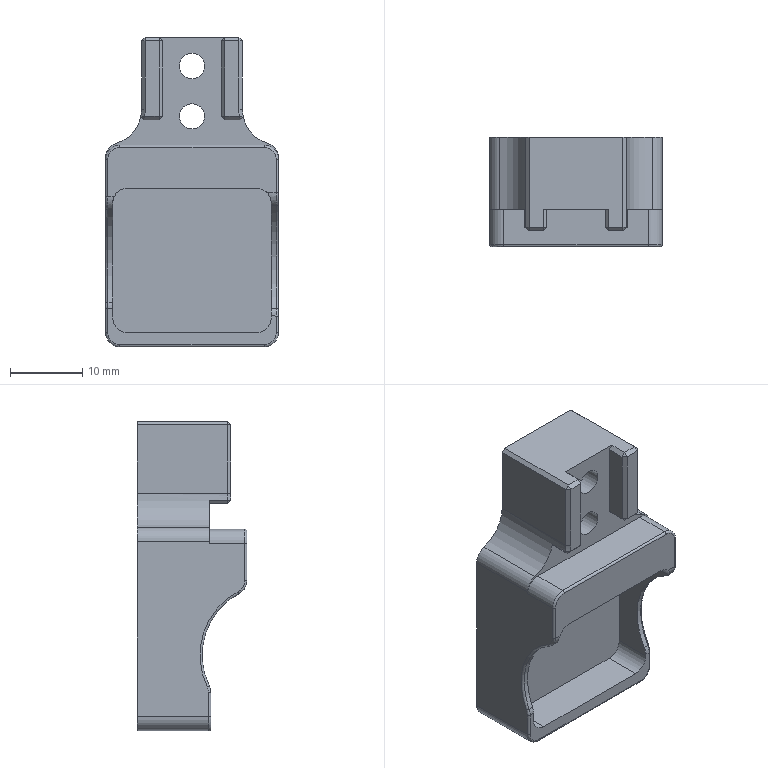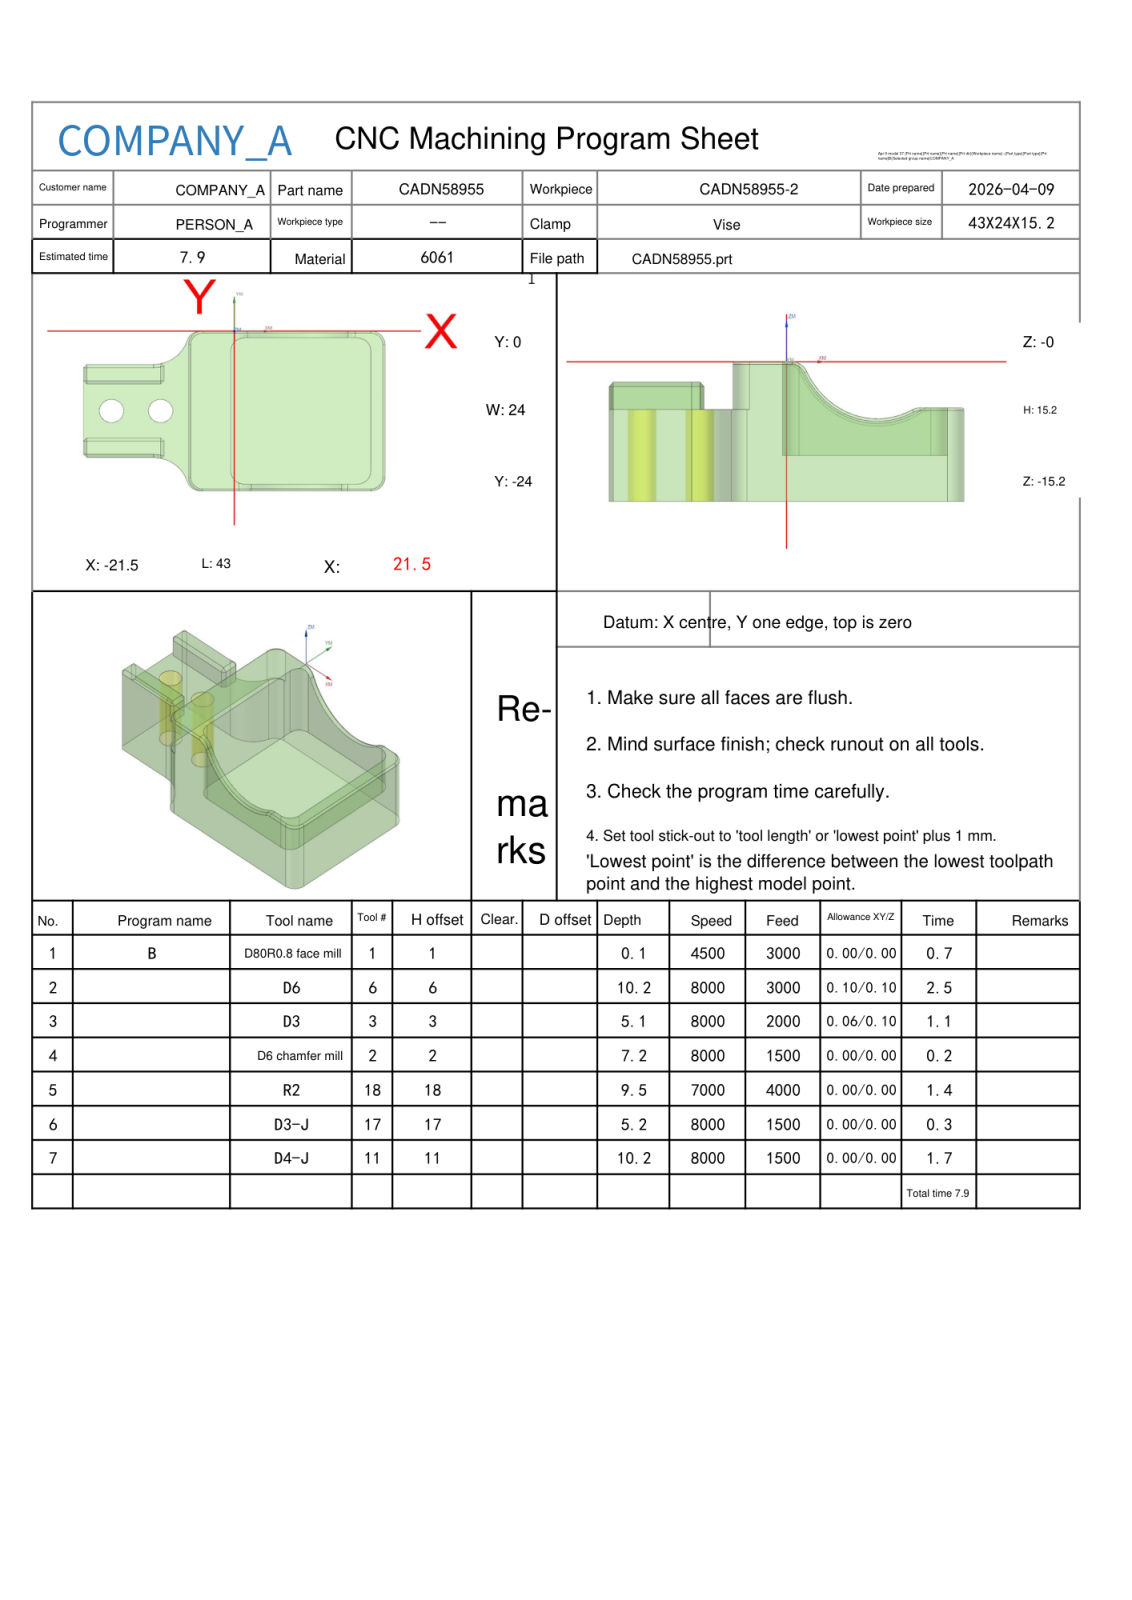NC program | NX | posted by the shop | part box 24 x 15.2 x 43 mm
Lines 1 to 2342 of 14472, first 1929 of 2340 lines:
%
O0001
(Machine time: 9.20 MIN)
(===Total Tool:7===)
(T1=D80R0.8 face mill D=80.  R=0.8  D-  H01 Z=-0.   )
(T6=D6      D=6.   R=0.   D-  H06 Z=-10.2 )
(T3=D3      D=3.   R=0.   D-  H03 Z=-5.1  )
(T2=D6 chamfer mill   D=6.   R=0.   D-  H02 Z=-7.25 )
(T18=R2     D=4.   R=2.   D-  H18 Z=-9.45 )
(T17=D3-J   D=3.   R=0.   D17 H17 Z=-5.2  )
(T11=D4-J   D=4.   R=0.   D11 H11 Z=-10.2 )
G80 G90 G17 G49 G40
G91 G28 Z0
M01
N1 T01 M06
(D80R0.8 face mill D=80. R=0.8 H=01 ce=0.20 di=0.10)
G00 G90 G54 X73.5 Y-12. M03 S4500
G43 H01 Z20.
M08
Z6.011
G01 Z4.011 F3000.
X61.5
X-61.5
X-73.5
Z6.011
G00 Z7.5
X73.5
Z5.522
G01 Z3.522
X61.5
X-61.5
X-73.5
Z5.522
G00 Z7.011
X73.5
Z5.033
G01 Z3.033
X61.5
X-61.5
X-73.5
Z5.033
G00 Z6.522
X73.5
Z4.544
G01 Z2.544
X61.5
X-61.5
X-73.5
Z4.544
G00 Z6.033
X73.5
Z4.056
G01 Z2.056
X61.5
X-61.5
X-73.5
Z4.056
G00 Z5.544
X73.5
Z3.567
G01 Z1.567
X61.5
X-61.5
X-73.5
Z3.567
G00 Z5.056
X73.5
Z3.078
G01 Z1.078
X61.5
X-61.5
X-73.5
Z3.078
G00 Z4.567
X73.5
Z2.589
G01 Z.589
X61.5
X-61.5
X-73.5
Z2.589
G00 Z4.078
X73.5
Z2.1
G01 Z.1
X61.5
X-61.5
X-73.5
Z2.1
G00 Z20.
G00 G90 X73.5 Y-12. M03 S4500
Z20.
Z2.
G01 Z0.0 F1000.
X61.5
X-61.5
X-73.5
Z2.
G00 Z20.
G91 G28 Z0.0
M05
M09
G91 G28 Z0.0
M01
N2 T06 M06
(D6  D=6. R=0. H=06 ce=0.10 di=0.10)
G00 G90 G54 X-23.1 Y.5 M03 S8000
G43 H06 Z14.5
M08
Z1.32
G01 Z-.18 F3000.
Y-2.56
Y-20.84
G03 X-22.5 Y-21.44 I.6 J0.0
G01 X-19.2
G03 X-18.6 Y-20.84 I0.0 J.6
G01 Y-3.16
G02 X-18. Y-2.56 I.6 J0.0
G01 X-14.7
G02 X-14.1 Y-3.16 I0.0 J-.6
G01 Y-20.84
G03 X-13.5 Y-21.44 I.6 J0.0
G01 X-11.5
G02 X-11.034 Y-21.483 I0.0 J-2.56
G01 X-10.724 Y-22.04
G03 X-10.2 Y-22.348 I.524 J.292
X-9.6 Y-21.748 I0.0 J.6
G01 Y-2.252
Y4.261
Z1.32
G00 X-23.1 Y.5
Z.84
G01 Z-.66
Y-2.56
Y-20.84
G03 X-22.5 Y-21.44 I.6 J0.0
G01 X-19.2
G03 X-18.6 Y-20.84 I0.0 J.6
G01 Y-3.16
G02 X-18. Y-2.56 I.6 J0.0
G01 X-14.7
G02 X-14.1 Y-3.16 I0.0 J-.6
G01 Y-20.84
G03 X-13.5 Y-21.44 I.6 J0.0
G01 X-11.5
G02 X-11.034 Y-21.483 I0.0 J-2.56
G01 X-10.724 Y-22.04
G03 X-10.2 Y-22.348 I.524 J.292
X-9.6 Y-21.748 I0.0 J.6
G01 Y-2.252
Y4.293
Z.84
G00 X-23.1 Y.5
Z.36
G01 Z-1.14
Y-2.56
Y-20.84
G03 X-22.5 Y-21.44 I.6 J0.0
G01 X-19.2
G03 X-18.6 Y-20.84 I0.0 J.6
G01 Y-3.16
G02 X-18. Y-2.56 I.6 J0.0
G01 X-14.7
G02 X-14.1 Y-3.16 I0.0 J-.6
G01 Y-20.84
G03 X-13.5 Y-21.44 I.6 J0.0
G01 X-11.5
G02 X-11.034 Y-21.483 I0.0 J-2.56
G01 X-10.724 Y-22.04
G03 X-10.2 Y-22.348 I.524 J.292
X-9.6 Y-21.748 I0.0 J.6
G01 Y-2.252
Y4.293
Z.36
G00 X-23.1 Y.5
Z-.12
G01 Z-1.62
Y-2.56
Y-20.84
G03 X-22.5 Y-21.44 I.6 J0.0
G01 X-19.2
G03 X-18.6 Y-20.84 I0.0 J.6
G01 Y-3.16
G02 X-18. Y-2.56 I.6 J0.0
G01 X-14.7
G02 X-14.1 Y-3.16 I0.0 J-.6
G01 Y-20.84
G03 X-13.5 Y-21.44 I.6 J0.0
G01 X-11.5
G02 X-11.034 Y-21.483 I0.0 J-2.56
G01 X-10.724 Y-22.04
G03 X-10.2 Y-22.348 I.524 J.292
X-9.6 Y-21.748 I0.0 J.6
G01 Y-2.252
Y4.293
Z-.12
G00 X-23.1 Y.5
Z-.6
G01 Z-2.1
Y-2.56
Y-20.84
G03 X-22.5 Y-21.44 I.6 J0.0
G01 X-19.2
G03 X-18.6 Y-20.84 I0.0 J.6
G01 Y-3.16
G02 X-18. Y-2.56 I.6 J0.0
G01 X-14.7
G02 X-14.1 Y-3.16 I0.0 J-.6
G01 Y-20.84
G03 X-13.5 Y-21.44 I.6 J0.0
G01 X-11.5
G02 X-11.034 Y-21.483 I0.0 J-2.56
G01 X-10.724 Y-22.04
G03 X-10.2 Y-22.348 I.524 J.292
X-9.6 Y-21.748 I0.0 J.6
G01 Y-2.252
Y4.293
Z-.6
G00 Z14.5
G00 G90 X28.93 Y-7.803 M03 S8000
Z14.5
Z5.21
G01 Z4.01 F3000.
X28.499
G03 X24.299 Y-12.002 I0.0 J-4.2
G01 X24.297 Y-23.996
G02 X23.868 Y-24.798 I-4.925 J2.121
G01 X23.164 Y-24.8
X1.594 Y-24.798
Y-26.478
X1.595 Y-26.838
X.755 Y-26.839
X.754 Y-26.479
Y-23.719
X.734 Y-22.879
X.754 Y-22.876
X.829 Y-22.88
X.861 Y-22.81
X.81 Y-22.755
X.785 Y-22.715
X1.562 Y-21.053
X1.988 Y-20.803
X2.414 Y-20.579
X2.487 Y-20.558
X2.457 Y-20.488
X2.512 Y-20.469
X2.56 Y-20.476
X2.618 Y-20.508
X2.636 Y-20.445
X2.682 Y-20.38
X2.73 Y-20.255
X2.731 Y-20.048
X2.73 Y-19.928
Y-4.295
X2.732 Y-3.633
X2.796 Y-3.5
X2.814 Y-3.422
X2.735 Y-3.414
X2.654 Y-3.395
X2.637 Y-3.374
X2.623 Y-3.315
X2.569 Y-3.345
X2.58 Y-3.284
X2.518 Y-3.29
X2.462 Y-3.272
X2.397 Y-3.262
X1.551 Y-2.938
X.332 Y-1.642
X.381 Y-1.622
X.432 Y-1.548
X.362 Y-1.468
X.254 Y-1.457
X.208 Y-1.459
X.187 Y-.619
X.179 Y-.278
Y2.479
Y2.839
X1.019 Y2.838
Y2.479
Y.797
X23.891
G02 X24.299 Y.029 I-4.506 J-2.886
G01 X24.3 Y-.364
X24.298 Y-13.194
G02 X24.047 Y-13.682 I-.6 J0.0
G01 X20.349 Y-16.322
G03 X20.098 Y-16.81 I.349 J-.488
G01 Y-20.
G02 X19.498 Y-20.599 I-.6 J.001
G01 X7.53
G02 X6.931 Y-20.006 I.001 J.6
G01 X6.93 Y-19.907
Y-4.295
X6.938 Y-4.197
G03 X6.973 Y-3.939 I-4.221 J.706
G02 X7.569 Y-3.403 I.597 J-.064
G01 X19.5
G02 X20.1 Y-4.002 I-.001 J-.6
G01 X20.098 Y-13.146
G02 X19.787 Y-13.672 I-.6 J0.0
G01 X16.144 Y-15.666
G03 X15.865 Y-15.996 I.288 J-.526
G02 X15.299 Y-16.399 I-.567 J.196
G01 X11.729
G02 X11.13 Y-15.8 I.001 J.6
G01 Y-8.202
G02 X11.729 Y-7.603 I.6 J-.001
G01 X15.3
G02 X15.899 Y-8.202 I-.001 J-.6
G01 X15.898 Y-15.001
Y-15.501
G03 X20.098 Y-19.702 I4.2 J0.0
G01 X28.93 Y-19.703
Z5.21
G00 Z7.5
G01 Y-7.803 F6000.
G00 Z4.72
G01 Z3.52 F3000.
X28.499
G03 X24.299 Y-12.002 I0.0 J-4.2
G01 X24.297 Y-23.996
G02 X23.868 Y-24.798 I-4.925 J2.12
G01 X23.164 Y-24.8
X1.594 Y-24.799
Y-26.478
X1.595 Y-26.838
X.755 Y-26.839
X.754 Y-26.479
Y-23.719
X.734 Y-22.879
X.754 Y-22.876
X.829 Y-22.88
X.861 Y-22.81
X.81 Y-22.755
X.785 Y-22.715
X1.562 Y-21.053
X1.988 Y-20.803
X2.414 Y-20.579
X2.487 Y-20.558
X2.457 Y-20.488
X2.512 Y-20.469
X2.56 Y-20.476
X2.618 Y-20.508
X2.636 Y-20.445
X2.682 Y-20.38
X2.73 Y-20.255
X2.731 Y-20.049
X2.73 Y-19.928
Y-4.295
X2.732 Y-3.633
X2.796 Y-3.5
X2.814 Y-3.422
X2.735 Y-3.414
X2.654 Y-3.395
X2.637 Y-3.374
X2.623 Y-3.315
X2.569 Y-3.345
X2.58 Y-3.284
X2.518 Y-3.29
X2.462 Y-3.272
X2.397 Y-3.262
X1.551 Y-2.938
X.332 Y-1.642
X.381 Y-1.622
X.432 Y-1.548
X.362 Y-1.468
X.254 Y-1.457
X.208 Y-1.459
X.187 Y-.619
X.179 Y-.278
Y2.479
Y2.839
X1.019 Y2.838
Y2.479
Y.799
X23.164 Y.8
X23.89 Y.798
G02 X24.299 Y.029 I-4.506 J-2.887
G01 X24.3 Y-.364
X24.298 Y-15.002
G02 X23.841 Y-15.585 I-.6 J0.0
G01 X20.555 Y-16.39
G03 X20.098 Y-16.972 I.143 J-.583
G01 Y-20.001
G02 X19.499 Y-20.6 I-.6 J.001
G01 X7.53 Y-20.599
G02 X6.931 Y-20.006 I.001 J.6
G01 X6.93 Y-19.907
Y-4.295
X6.938 Y-4.197
G03 X6.973 Y-3.938 I-4.221 J.706
G02 X7.569 Y-3.401 I.597 J-.063
G01 X19.5 Y-3.4
G02 X20.1 Y-3.999 I-.001 J-.6
G01 X20.099 Y-13.146
G02 X19.787 Y-13.672 I-.6 J0.0
G01 X16.144 Y-15.666
G03 X15.865 Y-15.996 I.288 J-.526
G02 X15.299 Y-16.4 I-.567 J.196
G01 X11.729 Y-16.399
G02 X11.13 Y-15.8 I.001 J.6
G01 Y-8.2
G02 X11.729 Y-7.601 I.6 J-.001
G01 X15.3 Y-7.6
G02 X15.899 Y-8.2 I-.001 J-.6
G01 X15.898 Y-15.001
Y-15.501
G03 X20.098 Y-19.702 I4.2 J0.0
G01 X28.93 Y-19.703
Z4.72
G00 Z7.01
G01 Y-7.803 F6000.
G00 Z4.23
G01 Z3.03 F3000.
X28.499
G03 X24.299 Y-12.002 I0.0 J-4.2
G01 X24.297 Y-23.995
G02 X23.868 Y-24.798 I-4.925 J2.12
G01 X23.164 Y-24.8
X1.594 Y-24.799
Y-26.478
X1.595 Y-26.838
X.755 Y-26.839
X.754 Y-26.479
Y-23.719
X.734 Y-22.879
X.754 Y-22.876
X.829 Y-22.88
X.861 Y-22.81
X.81 Y-22.755
X.785 Y-22.715
X1.562 Y-21.053
X1.988 Y-20.803
X2.414 Y-20.579
X2.487 Y-20.558
X2.457 Y-20.488
X2.512 Y-20.469
X2.56 Y-20.476
X2.618 Y-20.508
X2.636 Y-20.445
X2.682 Y-20.38
X2.73 Y-20.255
X2.731 Y-20.049
X2.73 Y-19.928
Y-4.295
X2.732 Y-3.633
X2.796 Y-3.5
X2.814 Y-3.422
X2.735 Y-3.414
X2.654 Y-3.395
X2.637 Y-3.374
X2.623 Y-3.315
X2.569 Y-3.345
X2.58 Y-3.284
X2.518 Y-3.29
X2.462 Y-3.272
X2.397 Y-3.262
X1.551 Y-2.938
X.332 Y-1.642
X.381 Y-1.622
X.432 Y-1.548
X.362 Y-1.468
X.254 Y-1.457
X.208 Y-1.459
X.179 Y-.278
Y2.479
Y2.839
X1.019 Y2.838
Y2.479
Y.799
X23.164 Y.8
X23.89 Y.798
G02 X24.299 Y.029 I-4.506 J-2.887
G01 X24.3 Y-.364
X24.298 Y-15.002
G02 X23.841 Y-15.585 I-.6 J0.0
G01 X20.555 Y-16.39
G03 X20.098 Y-16.972 I.143 J-.583
G01 Y-20.001
G02 X19.499 Y-20.6 I-.6 J.001
G01 X7.53 Y-20.599
G02 X6.931 Y-20.006 I.001 J.6
G01 X6.93 Y-19.907
Y-4.295
X6.938 Y-4.197
G03 X6.973 Y-3.938 I-4.221 J.706
G02 X7.569 Y-3.401 I.597 J-.063
G01 X19.5 Y-3.4
G02 X20.1 Y-3.999 I-.001 J-.6
G01 X20.099 Y-13.146
G02 X19.787 Y-13.672 I-.6 J0.0
G01 X16.144 Y-15.666
G03 X15.865 Y-15.996 I.288 J-.526
G02 X15.299 Y-16.4 I-.567 J.196
G01 X11.729 Y-16.399
G02 X11.13 Y-15.8 I.001 J.6
G01 Y-8.2
G02 X11.729 Y-7.601 I.6 J-.001
G01 X15.3 Y-7.6
G02 X15.899 Y-8.2 I-.001 J-.6
G01 X15.898 Y-15.001
Y-15.501
G03 X20.098 Y-19.702 I4.2 J0.0
G01 X28.93 Y-19.703
Z4.23
G00 Z6.52
G01 Y-7.803 F6000.
G00 Z3.74
G01 Z2.54 F3000.
X28.499
G03 X24.299 Y-12.002 I0.0 J-4.2
G01 X24.297 Y-23.995
G02 X23.868 Y-24.798 I-4.925 J2.12
G01 X23.164 Y-24.8
X1.594 Y-24.799
Y-26.478
X1.595 Y-26.838
X.755 Y-26.839
X.754 Y-26.479
Y-23.719
X.734 Y-22.879
X.754 Y-22.876
X.829 Y-22.88
X.861 Y-22.81
X.81 Y-22.755
X.785 Y-22.715
X1.562 Y-21.053
X1.988 Y-20.803
X2.414 Y-20.579
X2.487 Y-20.558
X2.457 Y-20.488
X2.512 Y-20.469
X2.56 Y-20.476
X2.618 Y-20.508
X2.636 Y-20.445
X2.682 Y-20.38
X2.73 Y-20.255
X2.731 Y-20.049
X2.73 Y-19.928
Y-4.295
X2.732 Y-3.633
X2.796 Y-3.5
X2.814 Y-3.422
X2.735 Y-3.414
X2.654 Y-3.395
X2.637 Y-3.374
X2.623 Y-3.315
X2.569 Y-3.345
X2.58 Y-3.284
X2.518 Y-3.29
X2.462 Y-3.272
X2.397 Y-3.262
X1.551 Y-2.938
X.332 Y-1.642
X.381 Y-1.622
X.432 Y-1.548
X.362 Y-1.468
X.254 Y-1.457
X.208 Y-1.459
X.187 Y-.619
X.179 Y-.278
Y2.479
Y2.839
X1.019 Y2.838
Y2.479
Y.799
X23.164 Y.8
X23.89 Y.798
G02 X24.299 Y.029 I-4.506 J-2.887
G01 X24.3 Y-.364
X24.298 Y-15.002
G02 X23.841 Y-15.585 I-.6 J0.0
G01 X20.555 Y-16.39
G03 X20.098 Y-16.972 I.143 J-.583
G01 Y-20.001
G02 X19.499 Y-20.6 I-.6 J.001
G01 X7.53 Y-20.599
G02 X6.931 Y-20.006 I.001 J.6
G01 X6.93 Y-19.907
Y-4.295
X6.938 Y-4.197
G03 X6.973 Y-3.938 I-4.221 J.706
G02 X7.569 Y-3.401 I.597 J-.063
G01 X19.5 Y-3.4
G02 X20.1 Y-3.999 I-.001 J-.6
G01 X20.099 Y-13.146
G02 X19.787 Y-13.672 I-.6 J0.0
G01 X16.144 Y-15.666
G03 X15.865 Y-15.996 I.288 J-.526
G02 X15.299 Y-16.4 I-.567 J.196
G01 X11.729 Y-16.399
G02 X11.13 Y-15.8 I.001 J.6
G01 Y-8.2
G02 X11.729 Y-7.601 I.6 J-.001
G01 X15.3 Y-7.6
G02 X15.899 Y-8.2 I-.001 J-.6
G01 X15.898 Y-15.001
Y-15.501
G03 X20.098 Y-19.702 I4.2 J0.0
G01 X28.93 Y-19.703
Z3.74
G00 Z6.03
G01 Y-7.803 F6000.
G00 Z3.25
G01 Z2.05 F3000.
X28.499
G03 X24.299 Y-12.002 I0.0 J-4.2
G01 X24.298 Y-23.995
G02 X23.868 Y-24.798 I-4.926 J2.12
G01 X23.164 Y-24.8
X1.594 Y-24.799
Y-26.478
X1.595 Y-26.838
X.755 Y-26.839
X.754 Y-26.479
Y-23.719
X.734 Y-22.879
X.754 Y-22.876
X.829 Y-22.88
X.861 Y-22.81
X.81 Y-22.755
X.785 Y-22.715
X1.562 Y-21.053
X1.988 Y-20.803
X2.414 Y-20.579
X2.487 Y-20.558
X2.457 Y-20.488
X2.512 Y-20.469
X2.56 Y-20.476
X2.618 Y-20.508
X2.636 Y-20.445
X2.682 Y-20.38
X2.73 Y-20.255
X2.731 Y-20.049
X2.73 Y-19.928
Y-4.295
X2.732 Y-3.633
X2.796 Y-3.5
X2.814 Y-3.422
X2.735 Y-3.414
X2.654 Y-3.395
X2.637 Y-3.374
X2.623 Y-3.315
X2.569 Y-3.345
X2.58 Y-3.284
X2.518 Y-3.29
X2.462 Y-3.272
X2.397 Y-3.262
X1.551 Y-2.938
X.332 Y-1.642
X.381 Y-1.622
X.432 Y-1.548
X.362 Y-1.468
X.254 Y-1.457
X.208 Y-1.459
X.187 Y-.619
X.179 Y-.278
Y2.479
Y2.839
X1.019 Y2.838
Y2.479
Y.8
X23.164
X23.89 Y.798
G02 X24.299 Y.028 I-4.505 J-2.887
G01 X24.3 Y-.364
X24.299 Y-15.002
G02 X23.841 Y-15.585 I-.6 J0.0
G01 X20.555 Y-16.39
G03 X20.098 Y-16.972 I.143 J-.583
G01 Y-20.001
G02 X19.499 Y-20.6 I-.6 J.001
G01 X7.53 Y-20.599
G02 X6.931 Y-20.006 I.001 J.6
G01 X6.93 Y-19.907
Y-4.295
X6.938 Y-4.197
G03 X6.973 Y-3.937 I-4.221 J.706
G02 X7.569 Y-3.4 I.597 J-.063
G01 X19.501
G02 X20.1 Y-3.999 I-.001 J-.6
G01 X20.099 Y-13.147
G02 X19.787 Y-13.672 I-.6 J0.0
G01 X16.144 Y-15.666
G03 X15.865 Y-15.996 I.288 J-.526
G02 X15.299 Y-16.4 I-.567 J.196
G01 X11.729 Y-16.399
G02 X11.13 Y-15.8 I.001 J.6
G01 Y-8.199
G02 X11.729 Y-7.6 I.6 J-.001
G01 X15.3
G02 X15.899 Y-8.199 I-.001 J-.6
G01 Y-15.001
X15.898 Y-15.501
G03 X20.098 Y-19.702 I4.2 J0.0
G01 X28.93 Y-19.703
Z3.25
G00 Z5.54
G01 Y-7.802 F6000.
G00 Z2.76
G01 Z1.56 F3000.
X28.498
G03 X24.298 Y-12.002 I0.0 J-4.2
G01 Y-23.995
G02 X23.868 Y-24.798 I-4.926 J2.119
G01 X23.164 Y-24.8
X1.594 Y-24.799
Y-26.478
X1.595 Y-26.838
X.755 Y-26.839
X.754 Y-26.479
Y-23.719
X.734 Y-22.879
X.754 Y-22.876
X.829 Y-22.88
X.861 Y-22.81
X.81 Y-22.755
X.785 Y-22.715
X1.562 Y-21.053
X1.988 Y-20.803
X2.414 Y-20.579
X2.487 Y-20.558
X2.457 Y-20.488
X2.512 Y-20.469
X2.56 Y-20.476
X2.618 Y-20.508
X2.636 Y-20.445
X2.682 Y-20.38
X2.73 Y-20.255
X2.731 Y-20.049
X2.73 Y-19.928
Y-4.295
X2.732 Y-3.633
X2.796 Y-3.5
X2.814 Y-3.422
X2.735 Y-3.414
X2.654 Y-3.395
X2.637 Y-3.374
X2.623 Y-3.315
X2.569 Y-3.345
X2.58 Y-3.284
X2.518 Y-3.29
X2.462 Y-3.272
X2.397 Y-3.262
X1.551 Y-2.938
X.332 Y-1.642
X.381 Y-1.622
X.432 Y-1.548
X.362 Y-1.468
X.254 Y-1.457
X.208 Y-1.459
X.187 Y-.619
X.179 Y-.278
Y2.479
Y2.839
X1.019 Y2.838
Y2.479
Y.8
X23.164
X23.89 Y.798
G02 X24.298 Y.032 I-4.505 J-2.887
G01 Y-15.002
G02 X23.84 Y-15.585 I-.6 J0.0
G01 X20.555 Y-16.39
G03 X20.098 Y-16.973 I.143 J-.583
G01 Y-20.001
G02 X19.499 Y-20.6 I-.6 J.001
G01 X7.53 Y-20.599
G02 X6.931 Y-20.006 I.001 J.6
G01 X6.93 Y-19.907
Y-4.295
X6.938 Y-4.197
G03 X6.973 Y-3.937 I-4.221 J.706
G02 X7.569 Y-3.4 I.597 J-.063
G01 X19.499
G02 X20.098 Y-3.999 I-.001 J-.6
G01 Y-13.147
G02 X19.786 Y-13.673 I-.6 J0.0
G01 X16.143 Y-15.666
G03 X15.865 Y-15.996 I.288 J-.526
G02 X15.299 Y-16.4 I-.567 J.196
G01 X11.729 Y-16.399
G02 X11.13 Y-15.8 I.001 J.6
G01 Y-8.199
G02 X11.729 Y-7.6 I.6 J-.001
G01 X15.299
G02 X15.898 Y-8.199 I-.001 J-.6
G01 Y-15.002
Y-15.502
G03 X20.098 Y-19.702 I4.2 J0.0
G01 X28.93
Z2.76
G00 Z5.05
G01 Y-7.802 F6000.
G00 Z2.27
G01 Z1.07 F3000.
X28.498
G03 X24.298 Y-12.002 I0.0 J-4.2
G01 Y-23.994
G02 X23.868 Y-24.798 I-4.926 J2.119
G01 X23.164 Y-24.8
X1.594 Y-24.799
Y-26.478
X1.595 Y-26.838
X.755 Y-26.839
X.754 Y-26.479
Y-23.719
X.734 Y-22.879
X.754 Y-22.876
X.829 Y-22.88
X.861 Y-22.81
X.81 Y-22.755
X.785 Y-22.715
X1.562 Y-21.053
X1.988 Y-20.803
X2.414 Y-20.579
X2.487 Y-20.558
X2.457 Y-20.488
X2.512 Y-20.469
X2.56 Y-20.476
X2.618 Y-20.508
X2.636 Y-20.445
X2.682 Y-20.38
X2.73 Y-20.255
X2.731 Y-20.049
X2.73 Y-19.928
Y-4.295
X2.732 Y-3.633
X2.796 Y-3.5
X2.814 Y-3.422
X2.735 Y-3.414
X2.654 Y-3.395
X2.637 Y-3.374
X2.623 Y-3.315
X2.569 Y-3.345
X2.58 Y-3.284
X2.518 Y-3.29
X2.462 Y-3.272
X2.397 Y-3.262
X1.551 Y-2.938
X.332 Y-1.642
X.381 Y-1.622
X.432 Y-1.548
X.362 Y-1.468
X.254 Y-1.457
X.208 Y-1.459
X.187 Y-.619
X.179 Y-.278
Y2.479
Y2.839
X1.019 Y2.838
Y2.479
Y.8
X23.164
X23.89 Y.798
G02 X24.298 Y.031 I-4.505 J-2.887
G01 Y-15.002
G02 X23.841 Y-15.585 I-.6 J0.0
G01 X20.555 Y-16.39
G03 X20.098 Y-16.973 I.143 J-.583
G01 Y-20.001
G02 X19.499 Y-20.6 I-.6 J.001
G01 X7.53 Y-20.599
G02 X6.931 Y-20.006 I.001 J.6
G01 X6.93 Y-19.907
Y-4.295
X6.938 Y-4.197
G03 X6.973 Y-3.937 I-4.221 J.706
G02 X7.569 Y-3.4 I.597 J-.063
G01 X19.499
G02 X20.098 Y-3.999 I-.001 J-.6
G01 Y-13.147
G02 X19.786 Y-13.673 I-.6 J0.0
G01 X16.143 Y-15.666
G03 X15.865 Y-15.996 I.288 J-.526
G02 X15.299 Y-16.4 I-.567 J.196
G01 X11.729 Y-16.399
G02 X11.13 Y-15.8 I.001 J.6
G01 Y-8.199
G02 X11.729 Y-7.6 I.6 J-.001
G01 X15.299
G02 X15.898 Y-8.199 I-.001 J-.6
G01 Y-15.002
Y-15.502
G03 X20.098 Y-19.702 I4.2 J0.0
G01 X28.93
Z2.27
G00 Z4.56
G01 Y-7.802 F6000.
G00 Z1.78
G01 Z.58 F3000.
X28.498
G03 X24.298 Y-12.002 I0.0 J-4.2
G01 Y-23.994
G02 X23.868 Y-24.798 I-4.926 J2.119
G01 X23.164 Y-24.8
X1.594 Y-24.799
Y-26.478
X1.595 Y-26.838
X.755 Y-26.839
X.754 Y-26.479
Y-23.719
X.734 Y-22.879
X.754 Y-22.876
X.829 Y-22.88
X.861 Y-22.81
X.81 Y-22.755
X.785 Y-22.715
X1.562 Y-21.053
X1.988 Y-20.803
X2.414 Y-20.579
X2.487 Y-20.558
X2.457 Y-20.488
X2.512 Y-20.469
X2.56 Y-20.476
X2.618 Y-20.508
X2.636 Y-20.445
X2.682 Y-20.38
X2.73 Y-20.255
X2.731 Y-20.049
X2.73 Y-19.928
Y-4.295
X2.732 Y-3.633
X2.796 Y-3.5
X2.814 Y-3.422
X2.735 Y-3.414
X2.654 Y-3.395
X2.637 Y-3.374
X2.623 Y-3.315
X2.569 Y-3.345
X2.58 Y-3.284
X2.518 Y-3.29
X2.462 Y-3.272
X2.397 Y-3.262
X1.551 Y-2.938
X.332 Y-1.642
X.381 Y-1.622
X.432 Y-1.548
X.362 Y-1.468
X.254 Y-1.457
X.208 Y-1.459
X.187 Y-.619
X.179 Y-.278
Y2.479
Y2.839
X1.019 Y2.838
Y2.479
Y.8
X23.164
X23.89 Y.798
G02 X24.298 Y.031 I-4.505 J-2.887
G01 Y-15.002
G02 X23.841 Y-15.585 I-.6 J0.0
G01 X20.555 Y-16.39
G03 X20.098 Y-16.973 I.143 J-.583
G01 Y-20.001
G02 X19.499 Y-20.6 I-.6 J.001
G01 X7.53 Y-20.599
G02 X6.931 Y-20.006 I.001 J.6
G01 X6.93 Y-19.907
Y-4.295
X6.938 Y-4.197
G03 X6.973 Y-3.937 I-4.221 J.706
G02 X7.569 Y-3.4 I.597 J-.063
G01 X19.499
G02 X20.098 Y-3.999 I-.001 J-.6
G01 Y-13.147
G02 X19.786 Y-13.673 I-.6 J0.0
G01 X16.144 Y-15.666
G03 X15.865 Y-15.996 I.288 J-.526
G02 X15.299 Y-16.4 I-.567 J.196
G01 X11.729 Y-16.399
G02 X11.13 Y-15.8 I.001 J.6
G01 Y-8.199
G02 X11.729 Y-7.6 I.6 J-.001
G01 X15.299
G02 X15.898 Y-8.199 I-.001 J-.6
G01 Y-15.002
Y-15.502
G03 X20.098 Y-19.702 I4.2 J0.0
G01 X28.93
Z1.78
G00 Z4.07
G01 Y-7.802 F6000.
G00 Z1.29
G01 Z.09 F3000.
G03 X24.73 Y-12.002 I0.0 J-4.2
G01 Y-21.651
G02 X24.734 Y-21.875 I-5.358 J-.224
X19.372 Y-27.237 I-5.362 J0.0
X19.083 Y-27.23 I0.0 J5.362
G01 X1.681
X1.16
X.984
X.675 Y-27.229
X.59 Y-27.234
X.595 Y-27.15
Y-26.839
X.675
X.755
Y-26.831
G03 X3.979 Y-23.224 I-.405 J3.607
X2.655 Y-20.42 I-3.63 J0.0
G01 X2.682 Y-20.38
X2.73 Y-20.255
Y-19.928
X2.732 Y-3.633
X2.787 Y-3.529
X2.836 Y-3.477
X2.806 Y-3.411
X2.735 Y-3.414
X2.654 Y-3.395
X2.639 Y-3.376
G03 X3.51 Y-.951 I-2.94 J2.425
X.179 Y2.83 I-3.811 J0.0
G01 Y2.839
X.019
X.02 Y3.15
X.016 Y3.234
X.1 Y3.229
X8.287 Y3.23
X17.077
X17.693
X19.11 Y3.229
X19.522 Y3.225
X19.791 Y3.221
X20.498 Y3.133
X20.906 Y3.024
X21.201 Y2.944
G02 X24.736 Y-2.089 I-1.816 J-5.034
X24.73 Y-2.35 I-5.351 J0.0
G01 Y-10.194
G02 X24.479 Y-10.682 I-.6 J0.0
G01 X20.781 Y-13.323
G03 X20.53 Y-13.811 I.349 J-.488
G01 Y-21.739
X20.538 Y-21.881
G02 X19.376 Y-23.044 I-1.162 J0.0
G01 X19.196 Y-23.03
X8.741
G02 X8.145 Y-22.487 I.001 J.6
G03 X7.018 Y-19.121 I-7.795 J-.737
G02 X6.93 Y-18.807 I.511 J.314
G01 Y-4.532
G02 X6.984 Y-4.284 I.6 J-.001
G03 X7.689 Y-1.526 I-7.285 J3.333
G02 X8.287 Y-.97 I.598 J-.044
G01 X17.059
X17.693
X19.061
X19.538 Y-.979
X19.728 Y-1.009
X19.816 Y-1.032
X19.958 Y-1.091
G02 X20.54 Y-2.092 I-.569 J-1.001
G01 X20.53 Y-2.247
Y-10.194
G02 X20.279 Y-10.682 I-.6 J0.0
G01 X16.581 Y-13.323
G03 X16.33 Y-13.811 I.349 J-.488
G01 Y-18.231
G02 X15.731 Y-18.83 I-.6 J.001
G01 X11.949
G02 X11.399 Y-18.468 I.001 J.6
G03 X11.189 Y-18.005 I-11.05 J-4.756
G02 X11.13 Y-17.747 I.541 J.259
G01 Y-5.769
G02 X11.729 Y-5.17 I.6 J-.001
G01 X15.73
G02 X16.33 Y-5.769 I-.001 J-.6
G01 Y-12.002
Y-12.502
G03 X20.53 Y-16.702 I4.2 J0.0
G01 X28.93
Z1.29
G00 Z3.58
G01 Y-7.802 F6000.
G00 Z.8
G01 Z-.4 F3000.
X28.498
G03 X24.298 Y-12.002 I0.0 J-4.2
G01 Y-23.994
G02 X23.868 Y-24.798 I-4.926 J2.119
G01 X5.761 Y-24.799
G02 X3.961 Y-27.23 I-4.195 J1.223
G01 X1.681
X1.16
X.984
X.713
Y-27.15
X1.16
X1.962 Y-27.083
G03 X5.095 Y-23.576 I-.397 J3.507
X5.053 Y-23.031 I-3.53 J0.0
G01 Y-23.017
G03 X2.73 Y-19.968 I-3.162 J0.0
G01 Y-17.396
Y-3.823
G03 X4.556 Y-.877 I-1.464 J2.946
X4.501 Y-.279 I-3.29 J0.0
X2.377 Y2.825 I-3.416 J-.059
X.587 Y3.151 I-1.789 J-4.74
G01 X.471 Y3.15
X.139
Y3.229
X3.407 Y3.23
G02 X5.187 Y.799 I-2.322 J-3.568
G01 X23.89 Y.798
G02 X24.298 Y.031 I-4.506 J-2.887
G01 Y-15.002
G02 X23.841 Y-15.585 I-.6 J0.0
G01 X20.555 Y-16.39
G03 X20.098 Y-16.973 I.143 J-.583
G01 Y-19.999
G02 X19.499 Y-20.598 I-.6 J.001
G01 X9.258
G02 X8.704 Y-20.227 I.001 J.6
G03 X7.104 Y-17.818 I-6.813 J-2.79
G02 X6.93 Y-17.396 I.426 J.423
G01 Y-5.995
G02 X7.065 Y-5.617 I.6 J-.001
G03 X8.175 Y-3.769 I-5.799 J4.74
G02 X8.727 Y-3.402 I.553 J-.233
G01 X19.499
G02 X20.098 Y-4.001 I-.001 J-.6
G01 Y-13.147
G02 X19.786 Y-13.673 I-.6 J0.0
G01 X16.144 Y-15.665
G03 X15.865 Y-15.994 I.288 J-.526
G02 X15.299 Y-16.398 I-.567 J.196
G01 X11.729
G02 X11.13 Y-15.799 I.001 J.6
G01 Y-8.201
G02 X11.729 Y-7.602 I.6 J-.001
G01 X15.299
G02 X15.898 Y-8.201 I-.001 J-.6
G01 Y-15.002
Y-15.502
G03 X20.098 Y-19.702 I4.2 J0.0
G01 X28.93
Z.8
G00 Z3.09
G01 Y-7.802 F6000.
G00 Z.31
G01 Z-.89 F3000.
X28.498
G03 X24.298 Y-12.002 I0.0 J-4.2
G01 Y-23.994
G02 X23.868 Y-24.798 I-4.926 J2.119
G01 X6.198 Y-24.799
G02 X4.437 Y-27.23 I-4.235 J1.214
G01 X1.903
Y-27.15
X1.963
G03 X5.529 Y-23.585 I0.0 J3.565
X5.485 Y-23.031 I-3.565 J0.0
G01 Y-23.015
G03 X2.73 Y-19.877 I-3.164 J0.0
G01 Y-4.
G03 X4.972 Y-.892 I-1.033 J3.108
X4.914 Y-.279 I-3.275 J0.0
X1.418 Y3.152 I-3.496 J-.066
G01 X1.31 Y3.15
Y3.229
X3.873 Y3.23
G02 X5.601 Y.799 I-2.453 J-3.574
G01 X23.89 Y.798
G02 X24.298 Y.031 I-4.506 J-2.887
G01 Y-15.002
G02 X23.841 Y-15.585 I-.6 J0.0
G01 X20.555 Y-16.39
G03 X20.098 Y-16.973 I.143 J-.583
G01 Y-19.999
G02 X19.499 Y-20.598 I-.6 J.001
G01 X9.691
G02 X9.137 Y-20.226 I.001 J.6
G03 X7.136 Y-17.443 I-6.816 J-2.788
G02 X6.93 Y-16.99 I.393 J.453
G01 Y-6.475
G02 X7.096 Y-6.062 I.6 J-.001
G03 X8.596 Y-3.77 I-5.399 J5.17
G02 X9.148 Y-3.402 I.553 J-.232
G01 X19.499
G02 X20.098 Y-4.001 I-.001 J-.6
G01 Y-13.147
G02 X19.786 Y-13.673 I-.6 J0.0
G01 X16.144 Y-15.665
G03 X15.865 Y-15.994 I.288 J-.526
G02 X15.299 Y-16.398 I-.567 J.196
G01 X12.112
G02 X11.631 Y-16.155 I.001 J.6
G03 X11.265 Y-15.684 I-9.31 J-6.86
G02 X11.13 Y-15.305 I.465 J.379
G01 Y-8.201
G02 X11.729 Y-7.602 I.6 J-.001
G01 X15.299
G02 X15.898 Y-8.201 I-.001 J-.6
G01 Y-15.002
Y-15.502
G03 X20.098 Y-19.702 I4.2 J0.0
G01 X28.93
Z.31
G00 Z2.6
G01 Y-7.802 F6000.
G00 Z-.18
G01 Z-1.38 F3000.
X28.498
G03 X24.298 Y-12.002 I0.0 J-4.2
G01 Y-23.994
G02 X23.868 Y-24.798 I-4.926 J2.119
G01 X6.475
G02 X4.752 Y-27.23 I-4.171 J1.13
G01 X2.234
Y-27.15
X2.275
X2.304
G03 X5.774 Y-23.949 I0.0 J3.482
X5.793 Y-23.476 I-5.853 J.472
X5.695 Y-22.406 I-5.872 J0.0
X2.73 Y-19.852 I-3.073 J-.57
G01 Y-4.078
G03 X5.043 Y-2.026 I-.609 J3.016
X5.241 Y-.796 I-3.727 J1.23
X5.207 Y-.279 I-3.924 J0.0
X1.709 Y3.15 I-3.498 J-.069
G01 X1.683
Y3.229
X4.163 Y3.23
G02 X5.893 Y.799 I-2.454 J-3.578
G01 X23.89 Y.798
G02 X24.298 Y.031 I-4.506 J-2.887
G01 Y-15.002
G02 X23.841 Y-15.585 I-.6 J0.0
G01 X20.555 Y-16.39
G03 X20.098 Y-16.973 I.143 J-.583
G01 Y-19.999
G02 X19.499 Y-20.598 I-.6 J.001
G01 X9.966
G02 X9.411 Y-20.225 I.001 J.6
G03 X7.157 Y-17.223 I-6.79 J-2.751
G02 X6.93 Y-16.754 I.372 J.47
G01 Y-6.787
G02 X7.117 Y-6.353 I.6 J-.001
G03 X8.873 Y-3.777 I-4.996 J5.291
G02 X9.428 Y-3.402 I.556 J-.225
G01 X19.499
G02 X20.098 Y-4.001 I-.001 J-.6
G01 Y-13.147
G02 X19.786 Y-13.673 I-.6 J0.0
G01 X16.144 Y-15.665
G03 X15.865 Y-15.994 I.288 J-.526
G02 X15.299 Y-16.398 I-.567 J.196
G01 X12.393
G02 X11.912 Y-16.154 I.001 J.6
G03 X11.278 Y-15.366 I-9.29 J-6.821
G02 X11.13 Y-14.972 I.452 J.395
G01 Y-8.377
G02 X11.252 Y-8.015 I.6 J-.001
G01 X11.378 Y-7.846
G02 X11.86 Y-7.602 I.483 J-.356
G01 X15.299
G02 X15.898 Y-8.201 I-.001 J-.6
G01 Y-15.002
Y-15.502
G03 X20.098 Y-19.702 I4.2 J0.0
G01 X28.93
Z-.18
G00 Z2.11
G01 Y-7.802 F6000.
G00 Z-.67
G01 Z-1.87 F3000.
X28.498
G03 X24.298 Y-12.002 I0.0 J-4.2
G01 Y-23.994
G02 X23.868 Y-24.798 I-4.926 J2.119
G01 X6.806
G02 X5.05 Y-27.23 I-4.225 J1.201
G01 X2.567
Y-27.15
X2.581
G03 X6.039 Y-24.41 I0.0 J3.552
G01 X6.104 Y-23.031
G03 X2.914 Y-19.85 I-3.208 J-.026
G01 X2.73
Y-19.01
Y-4.12
G03 X5.499 Y-1.313 I-.365 J3.129
G01 X5.534 Y-.969
G03 X5.549 Y-.619 I-4.211 J.349
X4.795 Y1.789 I-4.225 J0.0
X1.9 Y3.154 I-2.938 J-2.48
G01 X1.901 Y3.229
X4.422 Y3.23
G02 X5.485 Y2.268 I-2.573 J-3.915
X6.186 Y.798 I-4.161 J-2.887
G01 X23.89
G02 X24.298 Y.031 I-4.506 J-2.887
G01 Y-15.002
G02 X23.841 Y-15.585 I-.6 J0.0
G01 X20.555 Y-16.39
G03 X20.098 Y-16.973 I.143 J-.583
G01 Y-19.999
G02 X19.499 Y-20.598 I-.6 J.001
G01 X10.296
G02 X9.743 Y-20.229 I.001 J.6
G03 X7.182 Y-17.015 I-6.846 J-2.829
G02 X6.93 Y-16.527 I.348 J.489
G01 Y-7.034
G02 X7.139 Y-6.58 I.6 J-.001
G03 X9.168 Y-3.773 I-4.774 J5.589
G02 X9.722 Y-3.402 I.555 J-.228
G01 X19.499
G02 X20.098 Y-4.001 I-.001 J-.6
G01 Y-13.147
G02 X19.786 Y-13.673 I-.6 J0.0
G01 X16.144 Y-15.665
G03 X15.865 Y-15.995 I.288 J-.526
G02 X15.299 Y-16.398 I-.567 J.197
G01 X12.71
G02 X12.23 Y-16.156 I.001 J.6
G03 X11.295 Y-15.044 I-9.333 J-6.902
G02 X11.13 Y-14.632 I.435 J.413
G01 Y-8.731
G02 X11.266 Y-8.351 I.6 J-.001
G03 X11.662 Y-7.845 I-8.901 J7.36
G02 X12.143 Y-7.602 I.482 J-.357
G01 X15.299
G02 X15.898 Y-8.201 I-.001 J-.6
G01 Y-15.002
Y-15.502
G03 X20.098 Y-19.702 I4.2 J0.0
G01 X28.93
Z-.67
G00 Z1.62
G01 Y-7.802 F6000.
G00 Z-1.16
G01 Z-2.36 F3000.
X28.498
G03 X24.298 Y-12.002 I0.0 J-4.2
G01 Y-23.994
G02 X23.868 Y-24.798 I-4.926 J2.119
G01 X7.141
G02 X5.402 Y-27.23 I-4.203 J1.169
G01 X2.84
Y-27.151
X2.938 Y-27.152
G03 X6.414 Y-24.203 I0.0 J3.522
X6.473 Y-23.481 I-4.378 J.722
X6.45 Y-23.031 I-4.438 J0.0
G01 X6.384 Y-22.342
G03 X3.258 Y-19.85 I-3.136 J-.728
G01 X2.913
X2.73
Y-4.148
G03 X5.557 Y-2.348 I-.104 J3.282
G01 X5.578 Y-2.293
G03 X5.853 Y-.799 I-3.924 J1.494
X5.84 Y-.47 I-4.199 J0.0
X5.821 Y-.271 I-4.189 J-.307
X3.533 Y2.917 I-3.394 J-.022
X2.282 Y3.159 I-1.483 J-4.303
G01 X2.286 Y3.229
X4.777 Y3.23
G02 X6.518 Y.798 I-2.35 J-3.522
G01 X23.89
G02 X24.298 Y.031 I-4.506 J-2.887
G01 Y-15.002
G02 X23.841 Y-15.585 I-.6 J0.0
G01 X20.555 Y-16.39
G03 X20.098 Y-16.973 I.143 J-.583
G01 Y-19.999
G02 X19.499 Y-20.598 I-.6 J.001
G01 X10.655
G02 X10.102 Y-20.229 I.001 J.6
G03 X7.208 Y-16.795 I-6.854 J-2.841
G02 X6.93 Y-16.29 I.321 J.507
G01 Y-7.291
G02 X7.165 Y-6.816 I.6 J-.001
G03 X9.39 Y-4.074 I-4.534 J5.954
G01 X9.461 Y-3.897
X9.503 Y-3.787
G02 X10.062 Y-3.402 I.56 J-.215
G01 X19.499
G02 X20.098 Y-4.001 I-.001 J-.6
G01 Y-13.147
G02 X19.786 Y-13.673 I-.6 J0.0
G01 X16.144 Y-15.665
G03 X15.865 Y-15.995 I.288 J-.526
G02 X15.299 Y-16.398 I-.567 J.197
G01 X13.067
G02 X12.587 Y-16.156 I.001 J.6
G03 X11.312 Y-14.704 I-9.339 J-6.913
G02 X11.13 Y-14.275 I.417 J.431
G01 Y-9.113
G02 X11.284 Y-8.712 I.6 J-.001
G03 X12. Y-7.842 I-8.654 J7.85
G02 X12.479 Y-7.602 I.48 J-.36
G01 X15.299
G02 X15.898 Y-8.201 I-.001 J-.6
G01 Y-15.002
Y-15.502
G03 X20.098 Y-19.702 I4.2 J0.0
G01 X28.93
Z-1.16
G00 Z1.13
G01 Y-7.802 F6000.
G00 Z-1.65
G01 Z-2.85 F3000.
X28.498
G03 X24.298 Y-12.002 I0.0 J-4.2
G01 Y-23.994
G02 X23.868 Y-24.798 I-4.926 J2.119
G01 X7.561
G02 X5.801 Y-27.23 I-4.234 J1.213
G01 X3.26
Y-27.15
X3.277
X3.327
G03 X6.795 Y-24.41 I0.0 J3.565
G01 X6.862 Y-23.031
G03 X5.206 Y-20.25 I-3.206 J-.025
X3.653 Y-19.849 I-1.553 J-2.806
G01 X3.57 Y-19.85
X2.73
Y-4.15
X3.038
G03 X5.161 Y-3.339 I-.026 J3.254
X6.255 Y-.843 I-2.305 J2.497
X6.207 Y-.279 I-3.398 J0.0
X2.671 Y3.152 I-3.537 J-.107
G01 X2.557 Y3.15
Y3.23
X5.138
G02 X6.886 Y.798 I-2.466 J-3.616
G01 X23.89
G02 X24.298 Y.031 I-4.506 J-2.887
G01 Y-15.002
G02 X23.841 Y-15.585 I-.6 J0.0
G01 X20.555 Y-16.39
G03 X20.098 Y-16.973 I.143 J-.583
G01 Y-19.999
G02 X19.499 Y-20.598 I-.6 J.001
G01 X11.053
G02 X10.501 Y-20.229 I.001 J.6
G03 X7.238 Y-16.574 I-6.845 J-2.828
G02 X6.93 Y-16.051 I.291 J.524
G01 Y-7.563
G02 X7.192 Y-7.068 I.6 J-.001
G03 X7.973 Y-6.46 I-4.179 J6.172
X9.868 Y-3.769 I-5.117 J5.617
G02 X10.42 Y-3.402 I.553 J-.232
G01 X19.499
G02 X20.098 Y-4.001 I-.001 J-.6
G01 Y-13.147
G02 X19.786 Y-13.673 I-.6 J0.0
G01 X16.144 Y-15.665
G03 X15.865 Y-15.995 I.288 J-.526
G02 X15.3 Y-16.398 I-.567 J.197
G01 X13.468
G02 X12.988 Y-16.156 I.001 J.6
G03 X11.332 Y-14.351 I-9.332 J-6.9
G02 X11.13 Y-13.904 I.398 J.449
G01 Y-9.5
G02 X11.299 Y-9.084 I.6 J-.001
G03 X12.352 Y-7.845 I-8.443 J8.241
G02 X12.833 Y-7.602 I.482 J-.357
G01 X15.3
G02 X15.898 Y-8.201 I-.002 J-.6
G01 Y-15.002
Y-15.502
G03 X20.098 Y-19.702 I4.2 J0.0
G01 X28.93
Z-1.65
G00 Z.64
G01 Y-7.802 F6000.
G00 Z-2.14
G01 Z-3.34 F3000.
X28.498
G03 X24.298 Y-12.002 I0.0 J-4.2
G01 Y-23.994
G02 X23.868 Y-24.798 I-4.926 J2.119
G01 X8.014
G02 X6.241 Y-27.23 I-4.256 J1.242
G01 X3.637
Y-27.15
X3.708
X3.758
G03 X7.352 Y-23.557 I0.0 J3.594
X7.313 Y-23.031 I-3.594 J0.0
X4.116 Y-19.85 I-3.21 J-.028
G01 X2.73
Y-4.15
X3.45
G03 X6.676 Y-.898 I-.026 J3.252
X6.617 Y-.279 I-3.252 J0.0
X5.948 Y1.676 I-3.55 J-.123
X3.063 Y3.152 I-2.884 J-2.078
G01 X2.93 Y3.15
Y3.23
X5.537
G02 X7.292 Y.798 I-2.471 J-3.632
G01 X23.89
G02 X24.298 Y.031 I-4.506 J-2.887
G01 Y-15.002
G02 X23.841 Y-15.585 I-.6 J0.0
G01 X20.555 Y-16.39
G03 X20.098 Y-16.973 I.143 J-.583
G01 Y-19.999
G02 X19.499 Y-20.598 I-.6 J.001
G01 X11.504
G02 X10.951 Y-20.229 I.001 J.6
G03 X7.272 Y-16.361 I-6.848 J-2.831
G02 X6.93 Y-15.821 I.258 J.542
G01 Y-7.823
G02 X7.223 Y-7.309 I.6 J-.001
G03 X10.301 Y-3.769 I-3.798 J6.411
G02 X10.853 Y-3.402 I.553 J-.233
G01 X19.499
G02 X20.098 Y-4.001 I-.001 J-.6
G01 Y-13.147
G02 X19.786 Y-13.673 I-.6 J0.0
G01 X16.143 Y-15.665
G03 X15.865 Y-15.995 I.288 J-.526
G02 X15.3 Y-16.398 I-.567 J.197
G01 X13.918
G02 X13.438 Y-16.156 I.002 J.6
G03 X11.354 Y-13.992 I-9.334 J-6.904
G02 X11.13 Y-13.526 I.376 J.468
G01 Y-9.904
G02 X11.322 Y-9.465 I.6 J-.002
G03 X12.78 Y-7.843 I-7.898 J8.567
G02 X13.26 Y-7.602 I.481 J-.359
G01 X15.3
G02 X15.898 Y-8.2 I-.002 J-.6
G01 Y-15.002
Y-15.502
G03 X20.098 Y-19.702 I4.2 J0.0
G01 X28.93
Z-2.14
G00 Z.15
G01 Y-7.802 F6000.
G00 Z-2.63
G01 Z-3.83 F3000.
X28.498
G03 X24.298 Y-12.002 I0.0 J-4.2
G01 Y-23.994
G02 X23.868 Y-24.798 I-4.926 J2.119
G01 X8.538
G02 X6.749 Y-27.23 I-4.286 J1.279
G01 X4.122
Y-27.15
X4.141
X4.252 Y-27.152
G03 X7.885 Y-23.519 I0.0 J3.632
X7.852 Y-23.031 I-3.632 J0.0
X4.638 Y-19.85 I-3.223 J-.042
G01 X2.731
X2.73
Y-19.01
Y-4.15
X3.918
G03 X7.163 Y-.891 I-.014 J3.259
X7.105 Y-.279 I-3.259 J0.0
G01 X7.098 Y-.173
G03 X3.517 Y3.151 I-3.582 J-.268
G01 X3.442 Y3.15
Y3.23
X6.
G02 X7.771 Y.798 I-2.483 J-3.671
G01 X23.89
G02 X24.298 Y.031 I-4.506 J-2.887
G01 Y-15.002
G02 X23.841 Y-15.585 I-.6 J0.0
G01 X20.555 Y-16.39
G03 X20.098 Y-16.973 I.143 J-.583
G01 Y-19.999
G02 X19.5 Y-20.598 I-.6 J.001
G01 X12.038
G02 X11.486 Y-20.229 I.001 J.6
G03 X7.311 Y-16.152 I-6.857 J-2.844
G02 X6.93 Y-15.594 I.218 J.559
G01 Y-8.087
G02 X7.259 Y-7.553 I.6 J-.002
G03 X10.785 Y-3.769 I-3.354 J6.662
G02 X11.337 Y-3.402 I.553 J-.233
G01 X19.5
G02 X20.098 Y-4.001 I-.002 J-.6
G01 Y-13.147
G02 X19.786 Y-13.673 I-.6 J0.0
G01 X16.143 Y-15.665
G03 X15.865 Y-15.995 I.288 J-.526
G02 X15.3 Y-16.398 I-.567 J.197
G01 X14.449
G02 X13.97 Y-16.156 I.002 J.6
G03 X11.38 Y-13.612 I-9.341 J-6.917
G02 X11.13 Y-13.126 I.35 J.487
G01 Y-10.326
G02 X11.345 Y-9.866 I.6 J-.002
G03 X13.264 Y-7.843 I-7.441 J8.975
G02 X13.743 Y-7.602 I.481 J-.359
G01 X15.3
G02 X15.898 Y-8.2 I-.002 J-.6
G01 Y-15.002
Y-15.502
G03 X20.098 Y-19.702 I4.2 J0.0
G01 X28.93
Z-2.63
G00 Z-.34
G01 Y-7.802 F6000.
G00 Z-3.12
G01 Z-4.32 F3000.
X28.498
G03 X24.298 Y-12.002 I0.0 J-4.2
G01 Y-23.994
G02 X23.868 Y-24.798 I-4.926 J2.119
G01 X9.182
G02 X7.38 Y-27.23 I-4.226 J1.249
G01 X4.774
X4.771 Y-27.147
G03 X5.858 Y-27.001 I-.206 J5.64
X8.522 Y-23.55 I-.903 J3.451
X8.484 Y-23.031 I-3.567 J0.0
X5.251 Y-19.85 I-3.233 J-.052
G01 X5.25
X2.73
Y-4.15
X4.471
G03 X7.628 Y-1.658 I-.013 J3.263
X7.717 Y-.768 I-4.421 J.89
X6.922 Y1.789 I-4.51 J0.0
X3.981 Y3.155 I-2.96 J-2.524
G01 X3.982 Y3.23
X6.541
G02 X7.614 Y2.265 I-2.59 J-3.958
X8.322 Y.798 I-4.407 J-3.033
G01 X23.89
G02 X24.298 Y.031 I-4.506 J-2.887
G01 Y-15.002
G02 X23.841 Y-15.585 I-.6 J0.0
G01 X20.555 Y-16.39
G03 X20.098 Y-16.973 I.143 J-.583
G01 Y-19.999
G02 X19.5 Y-20.598 I-.6 J.002
G01 X12.667
G02 X12.115 Y-20.23 I.002 J.6
G03 X7.358 Y-15.955 I-6.864 J-2.854
G02 X6.93 Y-15.381 I.172 J.575
G01 Y-8.34
G02 X7.3 Y-7.788 I.6 J-.002
G03 X11.342 Y-3.769 I-2.842 J6.9
G02 X11.893 Y-3.402 I.553 J-.233
G01 X19.5
G02 X20.098 Y-4.001 I-.002 J-.6
G01 Y-13.147
G02 X19.786 Y-13.673 I-.6 J0.0
G01 X16.143 Y-15.665
G03 X15.865 Y-15.995 I.288 J-.526
G02 X15.3 Y-16.398 I-.567 J.197
G01 X15.077
G02 X14.598 Y-16.157 I.002 J.6
G03 X11.411 Y-13.214 I-9.347 J-6.927
G02 X11.13 Y-12.708 I.319 J.508
G01 Y-10.759
G02 X11.373 Y-10.279 I.6 J-.002
G03 X13.819 Y-7.843 I-6.915 J9.391
G02 X14.298 Y-7.602 I.481 J-.359
G01 X15.3
G02 X15.898 Y-8.2 I-.002 J-.6
G01 Y-15.002
Y-15.502
G03 X20.098 Y-19.702 I4.2 J0.0
G01 X28.93
Z-3.12
G00 Z-.83
G01 Y-7.802 F6000.
G00 Z-3.61
G01 Z-4.81 F3000.
X28.498
G03 X24.298 Y-12.002 I0.0 J-4.2
G01 Y-23.994
G02 X23.868 Y-24.798 I-4.926 J2.119
G01 X9.945
G02 X8.128 Y-27.23 I-4.183 J1.231
G01 X5.362
Y-27.15
X5.442
G03 X7.1 Y-26.823 I-.105 J4.904
X9.283 Y-23.567 I-1.337 J3.256
X9.242 Y-23.031 I-3.52 J0.0
X6.003 Y-19.85 I-3.239 J-.058
G01 X5.985
X2.73
Y-4.15
X5.136
G03 X8.32 Y-1.264 I0.0 J3.2
G01 X8.35 Y-.969
G03 X8.369 Y-.586 I-3.718 J.383
X4.632 Y3.152 I-3.737 J0.0
G01 X4.522 Y3.15
Y3.23
X7.16
G02 X8.995 Y.798 I-2.527 J-3.815
G01 X23.89
G02 X24.298 Y.031 I-4.506 J-2.887
G01 Y-15.002
G02 X23.841 Y-15.585 I-.6 J0.0
G01 X20.555 Y-16.39
G03 X20.098 Y-16.973 I.143 J-.583
G01 Y-19.999
G02 X19.5 Y-20.598 I-.6 J.002
G01 X13.423
G02 X12.871 Y-20.23 I.002 J.6
G03 X7.414 Y-15.785 I-6.868 J-2.859
G02 X6.93 Y-15.198 I.115 J.589
G01 Y-8.582
G02 X7.349 Y-8.011 I.6 J-.002
G03 X11.977 Y-3.772 I-2.213 J7.061
G02 X12.529 Y-3.402 I.554 J-.23
G01 X19.5
G02 X20.098 Y-4.001 I-.002 J-.6
G01 Y-13.091
G02 X19.715 Y-13.651 I-.6 J0.0
G01 X16.195 Y-15.014
G03 X15.855 Y-15.35 I.217 J-.559
G02 X15.298 Y-15.727 I-.557 J.223
X14.843 Y-15.518 I0.0 J.6
G03 X11.447 Y-12.802 I-8.841 J-7.571
G02 X11.13 Y-12.274 I.282 J.529
G01 Y-11.213
G02 X11.404 Y-10.711 I.6 J-.002
G03 X14.465 Y-7.844 I-6.268 J9.76
G02 X14.945 Y-7.602 I.481 J-.358
G01 X15.3
G02 X15.898 Y-8.2 I-.002 J-.6
G01 Y-15.002
Y-15.129
G02 X15.784 Y-15.478 I-.6 J.002
G03 X14.989 Y-17.938 I3.404 J-2.46
X16.729 Y-21.342 I4.2 J0.0
G01 X26.416 Y-28.341
Z-3.61
G00 Z-1.32
G01 X20.246 Y-31.43 F6000.
G00 Z-4.1
G01 Z-5.3 F3000.
G03 X16.046 Y-27.23 I-4.2 J0.0
G01 X13.009
G02 X11.092 Y-24.798 I2.425 J3.883
G01 X10.916
G02 X9.065 Y-27.23 I-4.148 J1.238
G01 X6.066
Y-27.15
X6.182
X6.185
G03 X8.004 Y-26.823 I0.0 J5.226
X10.257 Y-23.56 I-1.235 J3.263
X10.217 Y-23.031 I-3.489 J0.0
X6.963 Y-19.85 I-3.254 J-.073
G01 X6.908
X2.73
Y-4.15
X5.871
X5.883
G03 X9.067 Y-1.658 I0.0 J3.281
X9.15 Y-.798 I-4.454 J.86
X8.34 Y1.789 I-4.536 J0.0
X5.29 Y3.152 I-3.05 J-2.732
G01 X5.255
Y3.23
X7.924
G02 X8.966 Y2.35 I-2.635 J-4.172
G01 X9.03 Y2.268
G02 X9.747 Y.798 I-4.416 J-3.066
G01 X12.254
G02 X14.054 Y3.23 I4.146 J-1.188
G01 X17.077
X17.693
X19.085
Y3.15
X17.23
G03 X16.985 Y3.155 I-.246 J-5.886
X15.604 Y2.991 I0.0 J-5.891
X12.929 Y-.279 I.796 J-3.381
X12.864 Y-.92 I3.166 J-.641
X16.094 Y-4.15 I3.23 J0.0
G01 X16.142
X16.35
Y-19.85
X15.099
X15.083
G03 X12.555 Y-20.963 I0.0 J-3.428
X11.696 Y-23.347 I2.879 J-2.384
X14.288 Y-26.905 I3.738 J0.0
X15.893 Y-27.157 I1.605 J4.982
X16.158 Y-27.15 I0.0 J5.234
G01 X19.083
Y-27.23
X17.56
X17.532 Y-27.229
X16.033 Y-27.156
X15.993
X15.893 Y-27.157
G02 X14.288 Y-26.905 I0.0 J5.234
X11.696 Y-23.347 I1.146 J3.558
X12.544 Y-20.977 I3.738 J0.0
G01 X12.567 Y-20.95
X12.632 Y-20.882
G03 X12.803 Y-20.463 I-.429 J.419
X12.688 Y-20.11 I-.6 J0.0
G01 X9.969 Y-16.377
G03 X9.705 Y-16.172 I-.485 J-.353
X7.486 Y-15.668 I-2.742 J-6.932
G02 X6.93 Y-15.071 I.044 J.598
G01 Y-8.779
G02 X7.406 Y-8.193 I.6 J-.002
G03 X10.619 Y-6.66 I-1.523 J7.324
G02 X10.997 Y-6.525 I.378 J-.466
X11.377 Y-6.661 I0.0 J-.6
G03 X11.891 Y-7.047 I4.717 J5.74
G02 X12.15 Y-7.539 I-.341 J-.494
G01 Y-15.849
G02 X11.809 Y-16.388 I-.6 J.002
G03 X11.249 Y-16.681 I3.245 J-6.907
G02 X11. Y-16.734 I-.248 J.546
X10.763 Y-16.686 I0.0 J.6
G01 Z-4.1
G00 Z1.62
G01 X3.143 Y7.43 F6000.
G00 Z-4.59
G01 Z-5.79 F3000.
G03 X7.343 Y3.23 I4.2 J0.0
G01 X8.834
G02 X9.909 Y2.373 I-2.749 J-4.55
G01 X9.985 Y2.282
G02 X10.731 Y.798 I-4.205 J-3.045
G01 X11.238
G02 X13.087 Y3.23 I4.093 J-1.193
G01 X15.89
X15.891 Y3.149
G03 X14.212 Y2.84 I.081 J-5.156
X11.91 Y-.279 I1.119 J-3.235
X11.851 Y-.898 I3.194 J-.619
X15.103 Y-4.151 I3.253 J0.0
G01 X15.174 Y-4.15
X16.35
Y-19.85
X13.836
X13.711 Y-19.848
G03 X10.991 Y-21.19 I0.0 J-3.427
X8.317 Y-19.85 I-2.674 J-1.997
G01 X2.73
Y-4.15
X6.812
X6.833
G03 X9.833 Y-2.348 I0.0 J3.398
X10.132 Y-.763 I-4.053 J1.584
X9.305 Y1.789 I-4.352 J0.0
X6.085 Y3.156 I-3.22 J-3.109
X5.853 Y3.15 I0.0 J-4.476
G01 Y3.23
X7.397 Y2.954
X7.478 Y2.934
G02 X9.271 Y1.824 I-1.393 J-4.253
G01 X9.333 Y1.749
G02 X10.132 Y-.763 I-3.553 J-2.513
X9.848 Y-2.31 I-4.352 J0.0
G01 X9.813 Y-2.384
G02 X9.614 Y-2.705 I-2.98 J1.632
G03 X9.505 Y-3.05 I.491 J-.345
X9.574 Y-3.329 I.6 J0.0
G01 X11.743 Y-7.447
G03 X11.911 Y-7.645 I.531 J.28
G02 X12.15 Y-8.123 I-.361 J-.479
G01 Y-15.338
G02 X11.709 Y-15.915 I-.6 J.002
G03 X11.199 Y-16.073 I2.002 J-7.359
G01 X11.003 Y-16.106
G02 X10.807 Y-16.073 I0.0 J.6
G03 X8.317 Y-15.65 I-2.49 J-7.114
G01 X7.528
G02 X6.93 Y-15.052 I.002 J.6
G01 Y-8.919
G02 X7.477 Y-8.323 I.6 J-.002
G03 X10.685 Y-7.301 I-.644 J7.57
G01 X10.8 Y-7.25
X10.988 Y-7.219
G02 X11.283 Y-7.297 I0.0 J-.6
G01 Z-4.59
G00 Z-.34
G01 X3.143 Y7.43 F6000.
G00 Z-5.08
G01 Z-6.28 F3000.
G03 X7.343 Y3.23 I4.2 J0.0
G01 X14.88
Y3.15
X14.846
X14.767 Y3.151
G03 X11.035 Y1.545 I0.0 J-5.139
G01 X10.998 Y1.504
X10.962 Y1.545
G03 X7.277 Y3.151 I-3.685 J-3.425
G01 X7.157 Y3.15
X7.045
Y3.23
X7.343
X7.843
G03 X12.043 Y7.43 I0.0 J4.2
G01 Z-5.08
G00 Z-2.79
G01 X6.727 F6000.
G00 Z-5.57
G01 Z-6.77 F3000.
G03 X10.927 Y3.23 I4.2 J0.0
G01 X13.486
Y3.15
X13.445
G02 X11.044 Y3.075 I-2.401 J38.639
X8.642 Y3.15 I0.0 J38.714
G01 X8.369
Y3.23
X10.927
X11.427
G03 X15.627 Y7.43 I0.0 J4.2
G01 Z-5.57
G00 Z-3.28
G01 X6.727 F6000.
G00 Z-6.06
G01 Z-7.26 F3000.
G03 X10.927 Y3.23 I4.2 J0.0